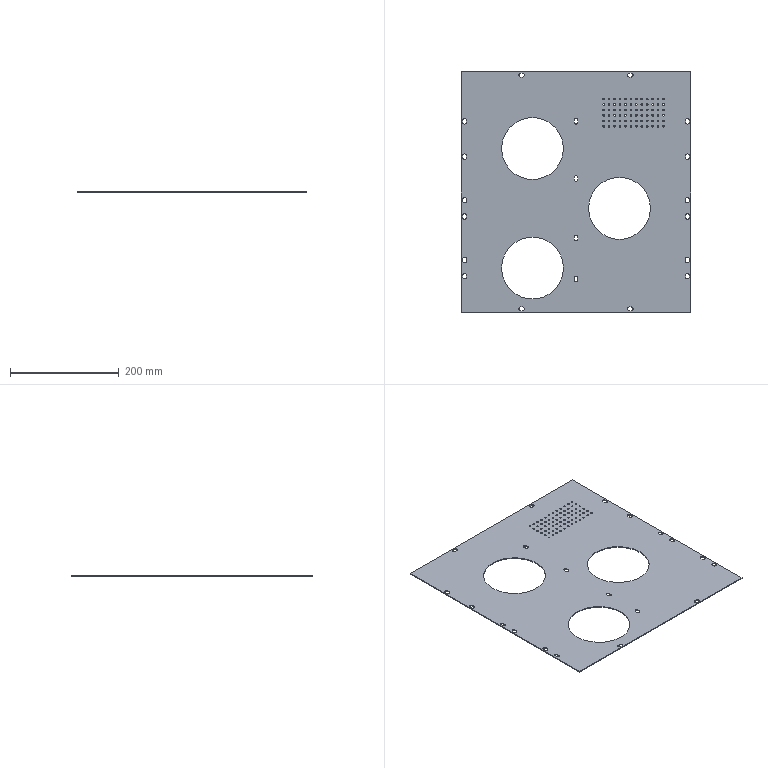Part | SolidWorks | features FlatPattern 1, SMBaseFlange 1, SheetMetal 1 | 1 solid | 240 faces | box 422 x 442 x 1.5 mm | volume 231306 mm3 | cylinder 194 | plane 46 | commonest cylinder face diameters 3 x144 7 x44 114 x6